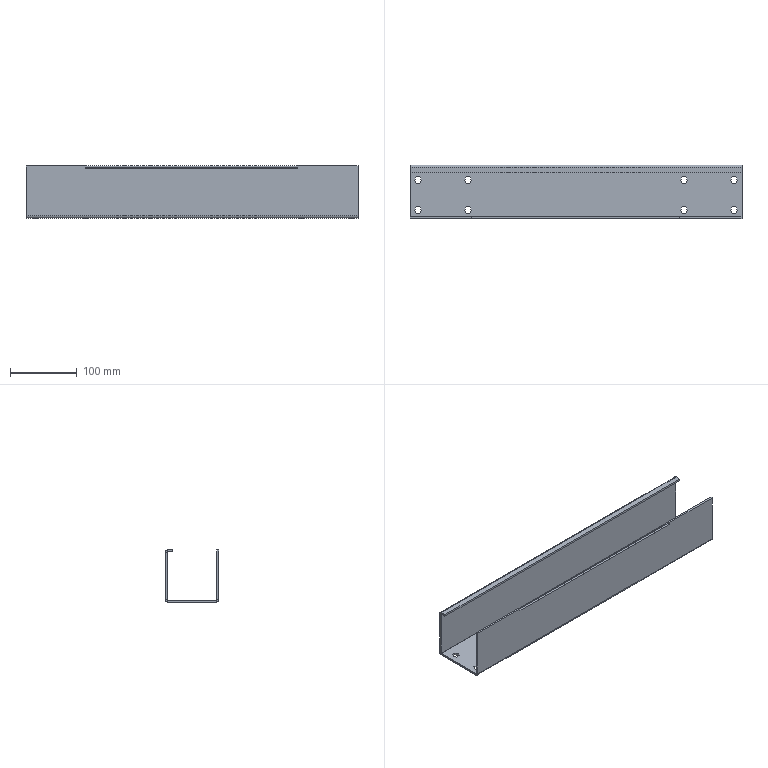Part | STEP file | 1 solid | 88 faces | box 498 x 80.2 x 78 mm | volume 347718 mm3 | plane 80 | cylinder 8 | commonest cylinder face diameters 0.4 x4 6.4 x4